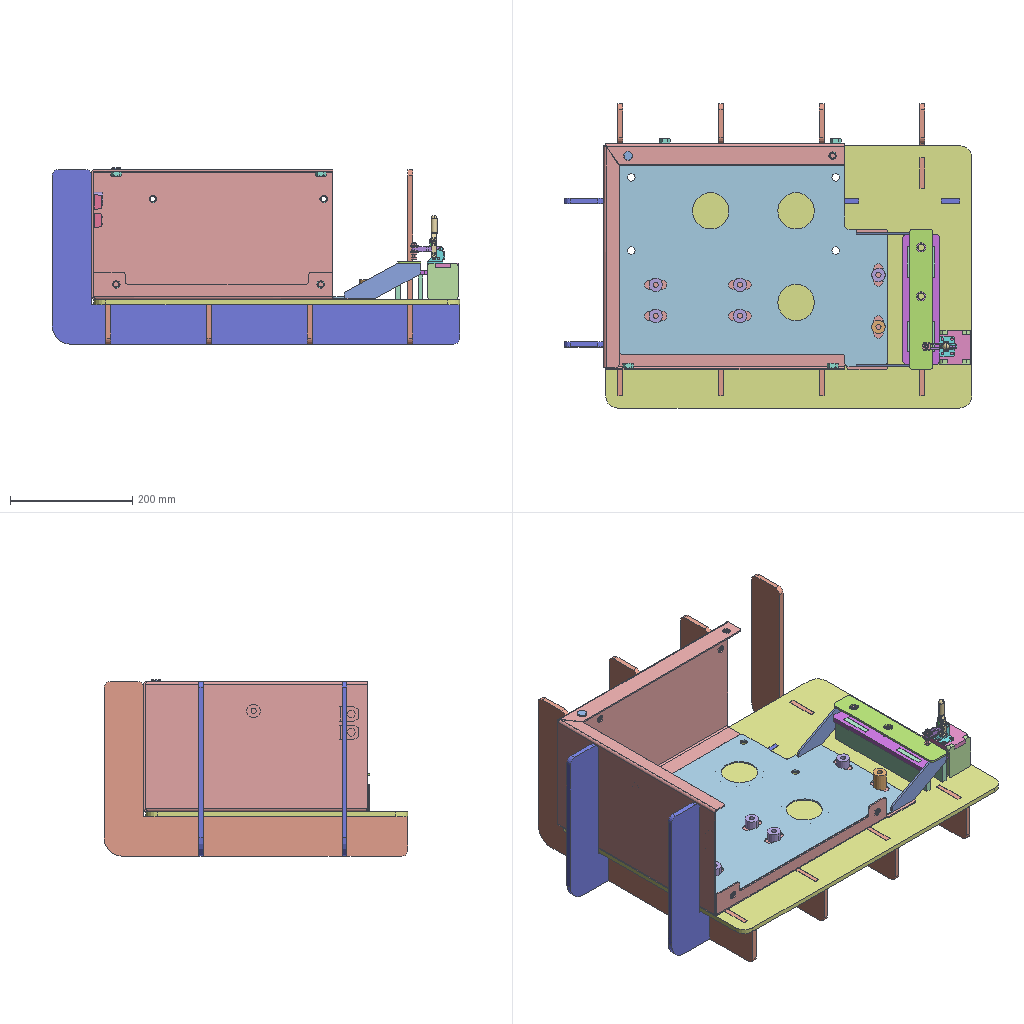Assembly | SolidWorks | 17 different items | 41 placed | box 668 x 498 x 289 mm
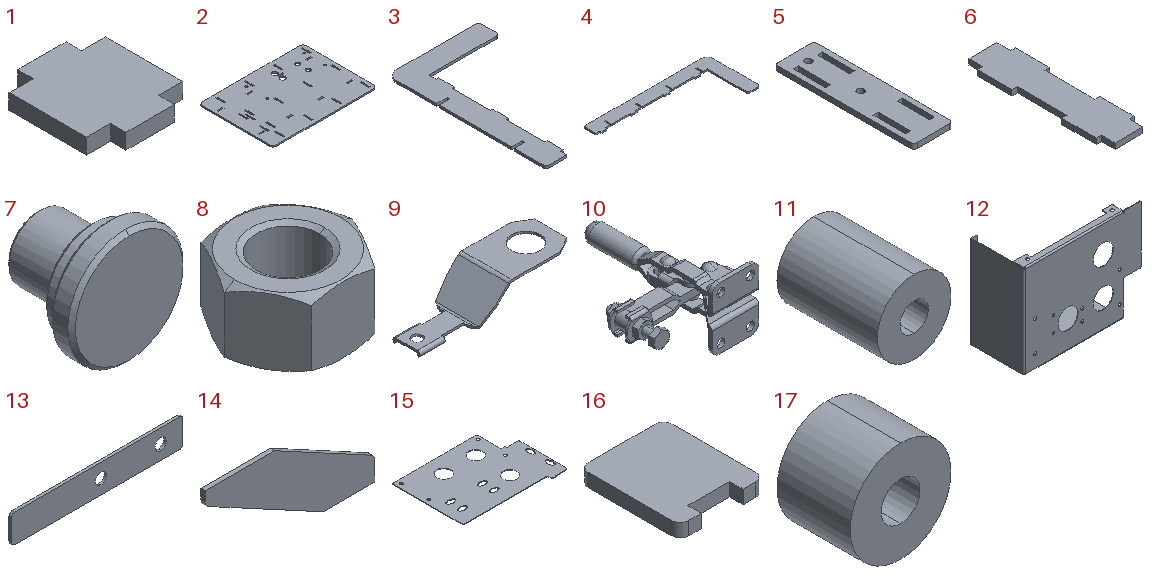Parts list (item | quantity | size | volume | features):
1 | x1 | 50 x 56 x 8 mm | 19200 mm3 | features FlatPattern 1, SMBaseFlange 1, SheetMetal 1
2 | x1 | 600 x 430 x 8 mm | 1971602 mm3 | features FlatPattern 1, SMBaseFlange 1, SheetMetal 1
3 | x4 | 286 x 498 x 8 mm | 376603 mm3 | features FlatPattern 1, SMBaseFlange 1, SheetMetal 1
4 | x2 | 668 x 286 x 8 mm | 459100 mm3 | features FlatPattern 1, SMBaseFlange 1, SheetMetal 1
5 | x1 | 60 x 212.5 x 8 mm | 87695 mm3 | features FlatPattern 1, SMBaseFlange 1, SheetMetal 1
6 | x2 | 55 x 212.5 x 8 mm | 80450 mm3 | features FlatPattern 1, SMBaseFlange 1, SheetMetal 1
7 | x1 | 15 x 12 x 15 mm | 1135 mm3 | features Chamfer 1, Revolution 1
8 | x12 | 27.713 x 24 x 14.8 mm | 5071 mm3 | features RevCut 2, Chamfer 1, Extrusion 1, LPattern 1
9 | x2 | 66.449 x 23 x 15.525 mm | 1224 mm3 | features ICE 6, EdgeFlange 2, Hem 2, FlatPattern 1, SMBaseFlange 1, SheetMetal 1
10 | x1 | 56.45 x 77.62 x 33.3 mm | 10418 mm3 | features BaseBody 5
11 | x1 | 22 x 30 x 22 mm | 9702 mm3 | features Extrusion 1, HoleWzd 1
12 | x1 | 465 x 213 x 370 mm | 766424 mm3 | features ICE 5, EdgeFlange 2, CornerRelief 1, Fillet 1, FlatPattern 1, SMBaseFlange 1, SheetMetal 1
13 | x1 | 230 x 3.2 x 38 mm | 26768 mm3 | features FlatPattern 1, SMBaseFlange 1, SheetMetal 1
14 | x2 | 125 x 3.2 x 57 mm | 11512 mm3 | features FlatPattern 1, SMBaseFlange 1, SheetMetal 1
15 | x1 | 440 x 330 x 2.3 mm | 269953 mm3 | features FlatPattern 1, SMBaseFlange 1, SheetMetal 1
16 | x2 | 50 x 60 x 8 mm | 22228 mm3 | features FlatPattern 1, SMBaseFlange 1, SheetMetal 1
17 | x6 | 22 x 16 x 22 mm | 5174 mm3 | features Extrusion 1, HoleWzd 1
Mates (type | each side: item.copy, entity, surface, feature):
Coincident | 12.1 face plane Base-Flange1 | 14.1 face plane Base-Flange1
DistanceDim | 14.1 face plane Base-Flange1 | 12.1 face plane Base-Flange1
Coincident | 12.1 face plane Base-Flange1 | 14.1 edge
Coincident | 14.2 face plane Base-Flange1 | 13.1 face plane Base-Flange1
Coincident | 12.1 face plane Base-Flange1 | 13.1 face plane Base-Flange1
Coincident | 14.2 edge | 13.1 edge
Coincident | 13.1 face plane Base-Flange1 | 8.1 face plane BaseNut
Concentric | 13.1 face cylinder Base-Flange1 | 8.1 edge
Parallel | 8.1 face plane BaseNut | assembly plane
Concentric | 13.1 face cylinder Base-Flange1 | 8.2 face cone EndChamfer
Coincident | 13.1 face plane Base-Flange1 | 8.2 face plane BaseNut
Parallel | 8.2 face plane BaseNut | assembly plane
Concentric | 12.1 face cylinder Cut-Extrude3 | 8.3 face cone EndChamfer
Coincident | 12.1 face plane Edge-Flange4 | 8.3 face plane BaseNut
Concentric | 12.1 face cylinder Cut-Extrude3 | 8.4 face cone EndChamfer
Coincident | 12.1 face plane Edge-Flange4 | 8.4 face plane BaseNut
Parallel | 12.1 face plane Edge-Flange4 | 8.3 face plane BaseNut
Parallel | 12.1 face plane Edge-Flange4 | 8.4 face plane BaseNut
Concentric | 12.1 face cylinder Cut-Extrude5 | 8.5 face cone EndChamfer
Coincident | 12.1 face plane Edge-Flange3 | 8.5 face plane BaseNut
Parallel | 8.5 face plane BaseNut | 12.1 face plane Edge-Flange4
Concentric | 12.1 face cylinder Cut-Extrude5 | 8.6 face cone EndChamfer
Coincident | 12.1 face plane Edge-Flange3 | 8.6 face plane BaseNut
Parallel | 12.1 face plane Edge-Flange4 | 8.6 face plane BaseNut
Concentric | 12.1 face cylinder Cut-Extrude4 | 8.7 face cone EndChamfer
Coincident | 12.1 face plane Edge-Flange3 | 8.7 face plane BaseNut
Parallel | 12.1 face plane Cut-Extrude1 | 8.7 face plane BaseNut
Concentric | 12.1 face cylinder Cut-Extrude4 | 8.8 face cone EndChamfer
Coincident | 12.1 face plane Edge-Flange3 | 8.8 face plane BaseNut
Parallel | 12.1 face plane Cut-Extrude1 | 8.8 face plane BaseNut
DistanceDim | 11.1 face cylinder Boss-Extrude1 | 12.1 face plane Edge-Flange3
Coincident | 12.1 face plane Base-Flange1 | 11.1 face plane Boss-Extrude1
Coincident | 12.1 face plane Base-Flange1 | 17.1 face plane Boss-Extrude1
DistanceDim | 17.1 face cylinder Boss-Extrude1 | 12.1 face plane Edge-Flange3 | 2 times
Concentric | 12.1 face cylinder Cut-Extrude2 | 8.9 face cone EndChamfer
Coincident | 12.1 face plane Base-Flange1 | 8.9 face plane BaseNut
Concentric | 12.1 face cylinder Cut-Extrude2 | 8.10 face cone EndChamfer
Coincident | 12.1 face plane Base-Flange1 | 8.10 face plane BaseNut
Parallel | 12.1 face plane Edge-Flange3 | 8.9 face plane BaseNut
Parallel | 12.1 face plane Edge-Flange3 | 8.10 face plane BaseNut
Concentric | 12.1 face cylinder Cut-Extrude2 | 8.11 face cone EndChamfer
Coincident | 12.1 face plane Base-Flange1 | 8.11 face plane BaseNut
Concentric | 12.1 face cylinder Cut-Extrude2 | 8.12 face cone EndChamfer
Coincident | 12.1 face plane Base-Flange1 | 8.12 face plane BaseNut
Parallel | 12.1 face plane Edge-Flange3 | 8.11 face plane BaseNut
Parallel | 12.1 face plane Edge-Flange3 | 8.12 face plane BaseNut
Coincident | 12.1 face plane Base-Flange1 | 17.2 face plane Boss-Extrude1
DistanceDim | 17.2 face cylinder Boss-Extrude1 | 12.1 face plane Edge-Flange3 | 2 times
DistanceDim | 11.1 face cylinder Boss-Extrude1 | 17.2 face cylinder Boss-Extrude1
Coincident | 12.1 face plane Edge-Flange3 | 17.3 face plane Boss-Extrude1
DistanceDim | 12.1 face plane Edge-Flange3 | 17.3 face cylinder Boss-Extrude1
DistanceDim | 12.1 face plane Base-Flange1 | 17.3 face cylinder Boss-Extrude1
Coincident | 12.1 face plane Edge-Flange3 | 9.1 face plane Base-Flange1
DistanceDim | 9.1 face cylinder Base-Flange1 | 12.1 face plane Edge-Flange3
DistanceDim | 12.1 face plane Base-Flange1 | 9.1 face cylinder Base-Flange1
InPlace | 12.1 face plane Base-Flange1 | 15.1 plane
InPlace | 12.1 face plane Base-Flange1 | 2.1 plane
InPlace | 5.1 plane | assembly plane
InPlace | 6.1 plane | assembly plane
InPlace | 3.1 plane | assembly plane
InPlace | 4.1 plane | assembly plane
InPlace | 5.1 face plane Base-Flange1 | 16.1 plane
InPlace | 16.1 face plane Base-Flange1 | 1.1 plane
Coincident | 1.1 face plane Base-Flange1 | 10.1 face plane TC1-1 vertical flange seat quick clamp [TCS1-1].step-1/_TCS1-1(seat).step-1-solid1 | 2 times
DistanceDim | 16.1 face plane Base-Flange1 | 10.1 face plane TC1-1 vertical flange seat quick clamp [TCS1-1].step-1/_TCS1-1(seat).step-1-solid1
InPlace | 7.1 plane | assembly plane